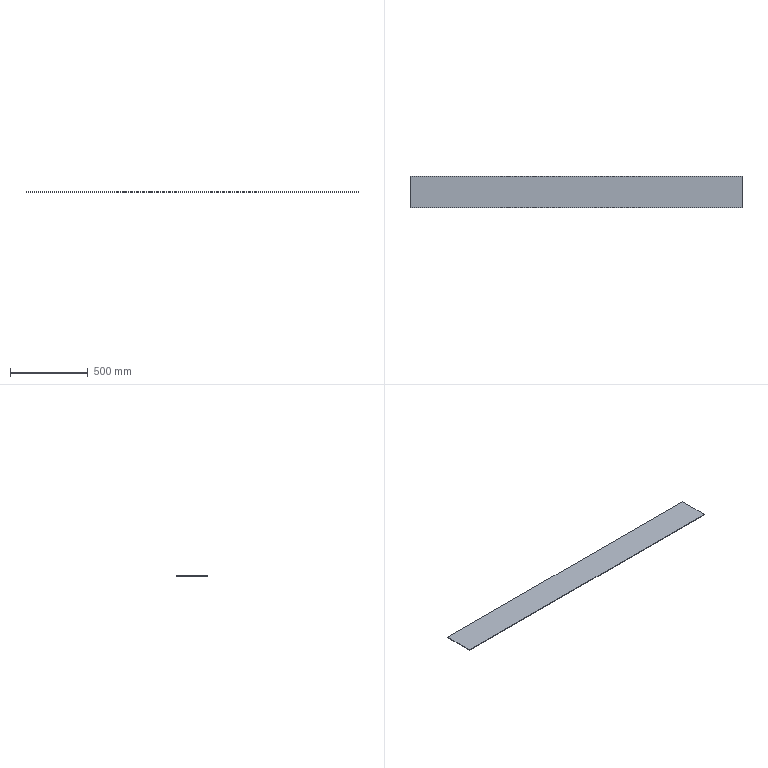Part | SolidWorks | features Extrusion 1, WeldmentFeature 1 | 1 solid | 6 faces | box 2140 x 200 x 4 mm | volume 1712000 mm3 | plane 6
STEP:
#1=CARTESIAN_POINT('',(-1070.,100.,0.));
#2=VERTEX_POINT('',#1);
#3=CARTESIAN_POINT('',(-1070.,-100.,0.));
#4=VERTEX_POINT('',#3);
#5=CARTESIAN_POINT('',(-1070.,-100.,0.));
#6=DIRECTION('',(0.,-1.,0.));
#7=VECTOR('',#6,1000.);
#8=LINE('',#5,#7);
#9=EDGE_CURVE('',#2,#4,#8,.T.);
#10=ORIENTED_EDGE('',*,*,#9,.T.);
#11=CARTESIAN_POINT('',(-1070.,-100.,4.));
#12=VERTEX_POINT('',#11);
#13=CARTESIAN_POINT('',(-1070.,-100.,4.));
#14=DIRECTION('',(0.,0.,-1.));
#15=VECTOR('',#14,1000.);
#16=LINE('',#13,#15);
#17=EDGE_CURVE('',#12,#4,#16,.T.);
#18=ORIENTED_EDGE('',*,*,#17,.F.);
#19=CARTESIAN_POINT('',(-1070.,100.,4.));
#20=VERTEX_POINT('',#19);
#21=CARTESIAN_POINT('',(-1070.,-100.,4.));
#22=DIRECTION('',(0.,-1.,0.));
#23=VECTOR('',#22,1000.);
#24=LINE('',#21,#23);
#25=EDGE_CURVE('',#20,#12,#24,.T.);
#26=ORIENTED_EDGE('',*,*,#25,.F.);
#27=CARTESIAN_POINT('',(-1070.,100.,4.));
#28=DIRECTION('',(0.,0.,-1.));
#29=VECTOR('',#28,1000.);
#30=LINE('',#27,#29);
#31=EDGE_CURVE('',#20,#2,#30,.T.);
#32=ORIENTED_EDGE('',*,*,#31,.T.);
#33=EDGE_LOOP('',(#10,#18,#26,#32));
#34=FACE_OUTER_BOUND('',#33,.T.);
#35=CARTESIAN_POINT('',(-1070.,-100.,4.));
#36=DIRECTION('',(1.,0.,0.));
#37=DIRECTION('',(0.,0.,-1.));
#38=AXIS2_PLACEMENT_3D('',#35,#36,#37);
#39=PLANE('',#38);
#40=ADVANCED_FACE('',(#34),#39,.F.);
#41=CARTESIAN_POINT('',(1070.,-100.,0.));
#42=VERTEX_POINT('',#41);
#43=CARTESIAN_POINT('',(1070.,-100.,0.));
#44=DIRECTION('',(1.,0.,0.));
#45=VECTOR('',#44,1000.);
#46=LINE('',#43,#45);
#47=EDGE_CURVE('',#4,#42,#46,.T.);
#48=ORIENTED_EDGE('',*,*,#47,.T.);
#49=CARTESIAN_POINT('',(1070.,-100.,4.));
#50=VERTEX_POINT('',#49);
#51=CARTESIAN_POINT('',(1070.,-100.,4.));
#52=DIRECTION('',(0.,0.,-1.));
#53=VECTOR('',#52,1000.);
#54=LINE('',#51,#53);
#55=EDGE_CURVE('',#50,#42,#54,.T.);
#56=ORIENTED_EDGE('',*,*,#55,.F.);
#57=CARTESIAN_POINT('',(1070.,-100.,4.));
#58=DIRECTION('',(1.,0.,0.));
#59=VECTOR('',#58,1000.);
#60=LINE('',#57,#59);
#61=EDGE_CURVE('',#12,#50,#60,.T.);
#62=ORIENTED_EDGE('',*,*,#61,.F.);
#63=ORIENTED_EDGE('',*,*,#17,.T.);
#64=EDGE_LOOP('',(#48,#56,#62,#63));
#65=FACE_OUTER_BOUND('',#64,.T.);
#66=CARTESIAN_POINT('',(1070.,-100.,4.));
#67=DIRECTION('',(0.,1.,0.));
#68=DIRECTION('',(-1.,0.,0.));
#69=AXIS2_PLACEMENT_3D('',#66,#67,#68);
#70=PLANE('',#69);
#71=ADVANCED_FACE('',(#65),#70,.F.);
#72=CARTESIAN_POINT('',(1070.,100.,0.));
#73=VERTEX_POINT('',#72);
#74=CARTESIAN_POINT('',(1070.,-100.,0.));
#75=DIRECTION('',(0.,1.,0.));
#76=VECTOR('',#75,1000.);
#77=LINE('',#74,#76);
#78=EDGE_CURVE('',#42,#73,#77,.T.);
#79=ORIENTED_EDGE('',*,*,#78,.T.);
#80=CARTESIAN_POINT('',(1070.,100.,4.));
#81=VERTEX_POINT('',#80);
#82=CARTESIAN_POINT('',(1070.,100.,4.));
#83=DIRECTION('',(0.,0.,-1.));
#84=VECTOR('',#83,1000.);
#85=LINE('',#82,#84);
#86=EDGE_CURVE('',#81,#73,#85,.T.);
#87=ORIENTED_EDGE('',*,*,#86,.F.);
#88=CARTESIAN_POINT('',(1070.,-100.,4.));
#89=DIRECTION('',(0.,1.,0.));
#90=VECTOR('',#89,1000.);
#91=LINE('',#88,#90);
#92=EDGE_CURVE('',#50,#81,#91,.T.);
#93=ORIENTED_EDGE('',*,*,#92,.F.);
#94=ORIENTED_EDGE('',*,*,#55,.T.);
#95=EDGE_LOOP('',(#79,#87,#93,#94));
#96=FACE_OUTER_BOUND('',#95,.T.);
#97=CARTESIAN_POINT('',(1070.,-100.,4.));
#98=DIRECTION('',(-1.,0.,0.));
#99=DIRECTION('',(0.,0.,1.));
#100=AXIS2_PLACEMENT_3D('',#97,#98,#99);
#101=PLANE('',#100);
#102=ADVANCED_FACE('',(#96),#101,.F.);
#103=CARTESIAN_POINT('',(1070.,100.,0.));
#104=DIRECTION('',(-1.,0.,0.));
#105=VECTOR('',#104,1000.);
#106=LINE('',#103,#105);
#107=EDGE_CURVE('',#73,#2,#106,.T.);
#108=ORIENTED_EDGE('',*,*,#107,.T.);
#109=ORIENTED_EDGE('',*,*,#31,.F.);
#110=CARTESIAN_POINT('',(1070.,100.,4.));
#111=DIRECTION('',(-1.,0.,0.));
#112=VECTOR('',#111,1000.);
#113=LINE('',#110,#112);
#114=EDGE_CURVE('',#81,#20,#113,.T.);
#115=ORIENTED_EDGE('',*,*,#114,.F.);
#116=ORIENTED_EDGE('',*,*,#86,.T.);
#117=EDGE_LOOP('',(#108,#109,#115,#116));
#118=FACE_OUTER_BOUND('',#117,.T.);
#119=CARTESIAN_POINT('',(1070.,100.,4.));
#120=DIRECTION('',(0.,-1.,0.));
#121=DIRECTION('',(1.,0.,0.));
#122=AXIS2_PLACEMENT_3D('',#119,#120,#121);
#123=PLANE('',#122);
#124=ADVANCED_FACE('',(#118),#123,.F.);
#125=ORIENTED_EDGE('',*,*,#25,.T.);
#126=ORIENTED_EDGE('',*,*,#61,.T.);
#127=ORIENTED_EDGE('',*,*,#92,.T.);
#128=ORIENTED_EDGE('',*,*,#114,.T.);
#129=EDGE_LOOP('',(#125,#126,#127,#128));
#130=FACE_OUTER_BOUND('',#129,.T.);
#131=CARTESIAN_POINT('',(0.,0.,4.));
#132=DIRECTION('',(0.,0.,1.));
#133=DIRECTION('',(1.,0.,0.));
#134=AXIS2_PLACEMENT_3D('',#131,#132,#133);
#135=PLANE('',#134);
#136=ADVANCED_FACE('',(#130),#135,.T.);
#137=ORIENTED_EDGE('',*,*,#9,.F.);
#138=ORIENTED_EDGE('',*,*,#107,.F.);
#139=ORIENTED_EDGE('',*,*,#78,.F.);
#140=ORIENTED_EDGE('',*,*,#47,.F.);
#141=EDGE_LOOP('',(#137,#138,#139,#140));
#142=FACE_OUTER_BOUND('',#141,.T.);
#143=CARTESIAN_POINT('',(0.,0.,0.));
#144=DIRECTION('',(0.,0.,1.));
#145=DIRECTION('',(1.,0.,0.));
#146=AXIS2_PLACEMENT_3D('',#143,#144,#145);
#147=PLANE('',#146);
#148=ADVANCED_FACE('',(#142),#147,.F.);
#149=CLOSED_SHELL('',(#40,#71,#102,#124,#136,#148));
#150=MANIFOLD_SOLID_BREP('',#149);
#151=CARTESIAN_POINT('',(0.,0.,0.));
#152=DIRECTION('',(0.,0.,1.));
#153=DIRECTION('',(1.,0.,0.));
#154=AXIS2_PLACEMENT_3D('',#151,#152,#153);
#155=(LENGTH_UNIT()NAMED_UNIT(*)SI_UNIT(.MILLI.,.METRE.));
#156=UNCERTAINTY_MEASURE_WITH_UNIT(LENGTH_MEASURE(0.00001),#155,'','');
#157=(NAMED_UNIT(*)PLANE_ANGLE_UNIT()SI_UNIT($,.RADIAN.));
#158=(NAMED_UNIT(*)SI_UNIT($,.STERADIAN.)SOLID_ANGLE_UNIT());
#159=(GEOMETRIC_REPRESENTATION_CONTEXT(3)GLOBAL_UNCERTAINTY_ASSIGNED_CONTEXT((#156))GLOBAL_UNIT_ASSIGNED_CONTEXT((#155,#157,#158))REPRESENTATION_CONTEXT('',''));
#160=ADVANCED_BREP_SHAPE_REPRESENTATION('',(#150,#154),#159);